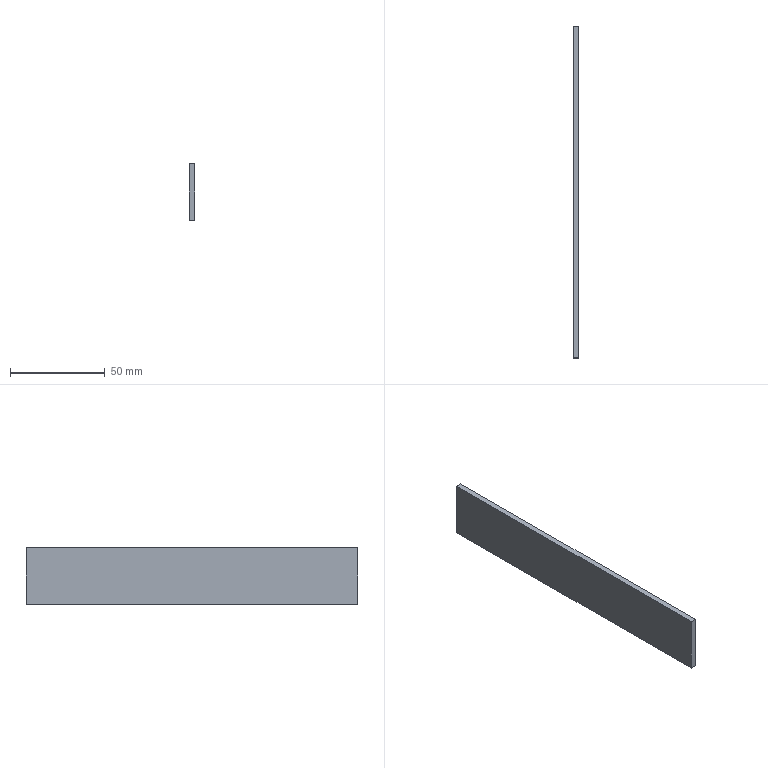Part | SolidWorks | 1 solid | 6 faces | box 3 x 175 x 30 mm | volume 15750 mm3 | plane 6
STEP:
#1=CARTESIAN_POINT('',(0.,87.5,15.));
#2=VERTEX_POINT('',#1);
#3=CARTESIAN_POINT('',(0.,-87.5,15.));
#4=VERTEX_POINT('',#3);
#5=CARTESIAN_POINT('',(0.,-87.5,15.));
#6=DIRECTION('',(0.,-1.,0.));
#7=VECTOR('',#6,1000.);
#8=LINE('',#5,#7);
#9=EDGE_CURVE('',#2,#4,#8,.T.);
#10=ORIENTED_EDGE('',*,*,#9,.F.);
#11=CARTESIAN_POINT('',(-3.,87.5,15.));
#12=VERTEX_POINT('',#11);
#13=CARTESIAN_POINT('',(-3.,87.5,15.));
#14=DIRECTION('',(1.,0.,0.));
#15=VECTOR('',#14,1000.);
#16=LINE('',#13,#15);
#17=EDGE_CURVE('',#12,#2,#16,.T.);
#18=ORIENTED_EDGE('',*,*,#17,.F.);
#19=CARTESIAN_POINT('',(-3.,-87.5,15.));
#20=VERTEX_POINT('',#19);
#21=CARTESIAN_POINT('',(-3.,-87.5,15.));
#22=DIRECTION('',(0.,-1.,0.));
#23=VECTOR('',#22,1000.);
#24=LINE('',#21,#23);
#25=EDGE_CURVE('',#12,#20,#24,.T.);
#26=ORIENTED_EDGE('',*,*,#25,.T.);
#27=CARTESIAN_POINT('',(-3.,-87.5,15.));
#28=DIRECTION('',(1.,0.,0.));
#29=VECTOR('',#28,1000.);
#30=LINE('',#27,#29);
#31=EDGE_CURVE('',#20,#4,#30,.T.);
#32=ORIENTED_EDGE('',*,*,#31,.T.);
#33=EDGE_LOOP('',(#10,#18,#26,#32));
#34=FACE_OUTER_BOUND('',#33,.T.);
#35=CARTESIAN_POINT('',(-3.,-87.5,15.));
#36=DIRECTION('',(0.,0.,1.));
#37=DIRECTION('',(1.,0.,0.));
#38=AXIS2_PLACEMENT_3D('',#35,#36,#37);
#39=PLANE('',#38);
#40=ADVANCED_FACE('',(#34),#39,.T.);
#41=CARTESIAN_POINT('',(0.,87.5,-15.));
#42=VERTEX_POINT('',#41);
#43=CARTESIAN_POINT('',(0.,87.5,-15.));
#44=DIRECTION('',(0.,0.,1.));
#45=VECTOR('',#44,1000.);
#46=LINE('',#43,#45);
#47=EDGE_CURVE('',#42,#2,#46,.T.);
#48=ORIENTED_EDGE('',*,*,#47,.F.);
#49=CARTESIAN_POINT('',(-3.,87.5,-15.));
#50=VERTEX_POINT('',#49);
#51=CARTESIAN_POINT('',(-3.,87.5,-15.));
#52=DIRECTION('',(1.,0.,0.));
#53=VECTOR('',#52,1000.);
#54=LINE('',#51,#53);
#55=EDGE_CURVE('',#50,#42,#54,.T.);
#56=ORIENTED_EDGE('',*,*,#55,.F.);
#57=CARTESIAN_POINT('',(-3.,87.5,-15.));
#58=DIRECTION('',(0.,0.,1.));
#59=VECTOR('',#58,1000.);
#60=LINE('',#57,#59);
#61=EDGE_CURVE('',#50,#12,#60,.T.);
#62=ORIENTED_EDGE('',*,*,#61,.T.);
#63=ORIENTED_EDGE('',*,*,#17,.T.);
#64=EDGE_LOOP('',(#48,#56,#62,#63));
#65=FACE_OUTER_BOUND('',#64,.T.);
#66=CARTESIAN_POINT('',(-3.,87.5,-15.));
#67=DIRECTION('',(0.,1.,0.));
#68=DIRECTION('',(0.,0.,1.));
#69=AXIS2_PLACEMENT_3D('',#66,#67,#68);
#70=PLANE('',#69);
#71=ADVANCED_FACE('',(#65),#70,.T.);
#72=CARTESIAN_POINT('',(0.,-87.5,-15.));
#73=VERTEX_POINT('',#72);
#74=CARTESIAN_POINT('',(0.,-87.5,-15.));
#75=DIRECTION('',(0.,1.,0.));
#76=VECTOR('',#75,1000.);
#77=LINE('',#74,#76);
#78=EDGE_CURVE('',#73,#42,#77,.T.);
#79=ORIENTED_EDGE('',*,*,#78,.F.);
#80=CARTESIAN_POINT('',(-3.,-87.5,-15.));
#81=VERTEX_POINT('',#80);
#82=CARTESIAN_POINT('',(-3.,-87.5,-15.));
#83=DIRECTION('',(1.,0.,0.));
#84=VECTOR('',#83,1000.);
#85=LINE('',#82,#84);
#86=EDGE_CURVE('',#81,#73,#85,.T.);
#87=ORIENTED_EDGE('',*,*,#86,.F.);
#88=CARTESIAN_POINT('',(-3.,-87.5,-15.));
#89=DIRECTION('',(0.,1.,0.));
#90=VECTOR('',#89,1000.);
#91=LINE('',#88,#90);
#92=EDGE_CURVE('',#81,#50,#91,.T.);
#93=ORIENTED_EDGE('',*,*,#92,.T.);
#94=ORIENTED_EDGE('',*,*,#55,.T.);
#95=EDGE_LOOP('',(#79,#87,#93,#94));
#96=FACE_OUTER_BOUND('',#95,.T.);
#97=CARTESIAN_POINT('',(-3.,-87.5,-15.));
#98=DIRECTION('',(0.,0.,-1.));
#99=DIRECTION('',(-1.,0.,0.));
#100=AXIS2_PLACEMENT_3D('',#97,#98,#99);
#101=PLANE('',#100);
#102=ADVANCED_FACE('',(#96),#101,.T.);
#103=CARTESIAN_POINT('',(0.,-87.5,-15.));
#104=DIRECTION('',(0.,0.,-1.));
#105=VECTOR('',#104,1000.);
#106=LINE('',#103,#105);
#107=EDGE_CURVE('',#4,#73,#106,.T.);
#108=ORIENTED_EDGE('',*,*,#107,.F.);
#109=ORIENTED_EDGE('',*,*,#31,.F.);
#110=CARTESIAN_POINT('',(-3.,-87.5,-15.));
#111=DIRECTION('',(0.,0.,-1.));
#112=VECTOR('',#111,1000.);
#113=LINE('',#110,#112);
#114=EDGE_CURVE('',#20,#81,#113,.T.);
#115=ORIENTED_EDGE('',*,*,#114,.T.);
#116=ORIENTED_EDGE('',*,*,#86,.T.);
#117=EDGE_LOOP('',(#108,#109,#115,#116));
#118=FACE_OUTER_BOUND('',#117,.T.);
#119=CARTESIAN_POINT('',(-3.,-87.5,-15.));
#120=DIRECTION('',(0.,-1.,0.));
#121=DIRECTION('',(0.,0.,-1.));
#122=AXIS2_PLACEMENT_3D('',#119,#120,#121);
#123=PLANE('',#122);
#124=ADVANCED_FACE('',(#118),#123,.T.);
#125=ORIENTED_EDGE('',*,*,#25,.F.);
#126=ORIENTED_EDGE('',*,*,#61,.F.);
#127=ORIENTED_EDGE('',*,*,#92,.F.);
#128=ORIENTED_EDGE('',*,*,#114,.F.);
#129=EDGE_LOOP('',(#125,#126,#127,#128));
#130=FACE_OUTER_BOUND('',#129,.T.);
#131=CARTESIAN_POINT('',(-3.,0.,0.));
#132=DIRECTION('',(1.,0.,0.));
#133=DIRECTION('',(0.,0.,-1.));
#134=AXIS2_PLACEMENT_3D('',#131,#132,#133);
#135=PLANE('',#134);
#136=ADVANCED_FACE('',(#130),#135,.F.);
#137=ORIENTED_EDGE('',*,*,#9,.T.);
#138=ORIENTED_EDGE('',*,*,#107,.T.);
#139=ORIENTED_EDGE('',*,*,#78,.T.);
#140=ORIENTED_EDGE('',*,*,#47,.T.);
#141=EDGE_LOOP('',(#137,#138,#139,#140));
#142=FACE_OUTER_BOUND('',#141,.T.);
#143=CARTESIAN_POINT('',(0.,0.,0.));
#144=DIRECTION('',(1.,0.,0.));
#145=DIRECTION('',(0.,0.,-1.));
#146=AXIS2_PLACEMENT_3D('',#143,#144,#145);
#147=PLANE('',#146);
#148=ADVANCED_FACE('',(#142),#147,.T.);
#149=CLOSED_SHELL('',(#40,#71,#102,#124,#136,#148));
#150=MANIFOLD_SOLID_BREP('',#149);
#151=CARTESIAN_POINT('',(0.,0.,0.));
#152=DIRECTION('',(0.,0.,1.));
#153=DIRECTION('',(1.,0.,0.));
#154=AXIS2_PLACEMENT_3D('',#151,#152,#153);
#155=(LENGTH_UNIT()NAMED_UNIT(*)SI_UNIT(.MILLI.,.METRE.));
#156=UNCERTAINTY_MEASURE_WITH_UNIT(LENGTH_MEASURE(0.00001),#155,'','');
#157=(NAMED_UNIT(*)PLANE_ANGLE_UNIT()SI_UNIT($,.RADIAN.));
#158=(NAMED_UNIT(*)SI_UNIT($,.STERADIAN.)SOLID_ANGLE_UNIT());
#159=(GEOMETRIC_REPRESENTATION_CONTEXT(3)GLOBAL_UNCERTAINTY_ASSIGNED_CONTEXT((#156))GLOBAL_UNIT_ASSIGNED_CONTEXT((#155,#157,#158))REPRESENTATION_CONTEXT('',''));
#160=ADVANCED_BREP_SHAPE_REPRESENTATION('',(#150,#154),#159);